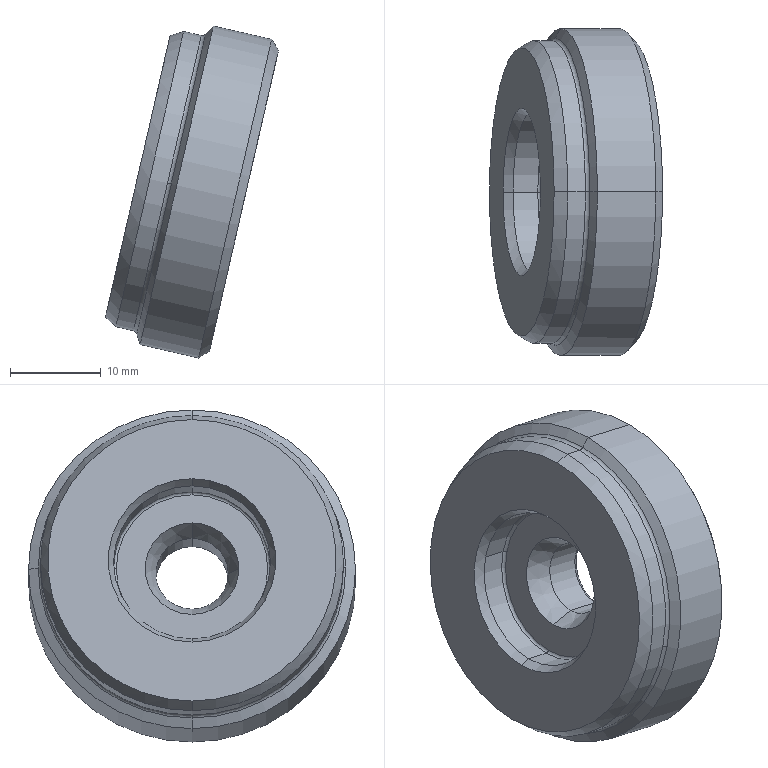Part | SolidWorks | features BaseBody 1 | 1 solid | 187 faces | box 19.061 x 36 x 36.564 mm | volume 8491 mm3 | plane 102 | cylinder 48 | torus 17 | cone 16 | spline 4 | commonest cylinder face diameters 0.5 x26 2 x13 17.3 x3 8 x2 33.36 x2 36 x2